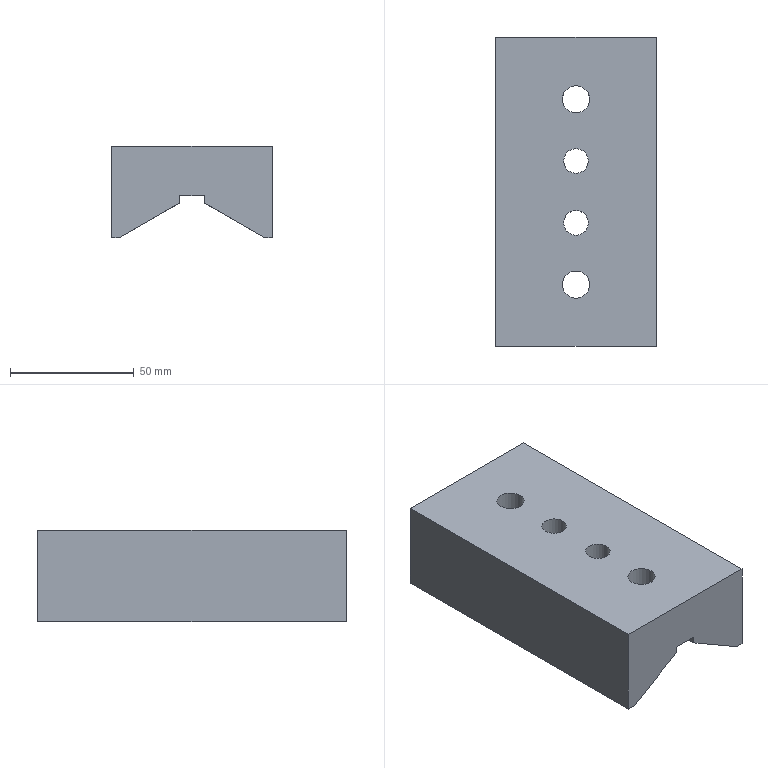Part | NX | features MAIN_BODY 2 | 1 solid | 34 faces | box 65 x 125 x 37 mm | volume 225809 mm3 | plane 24 | cylinder 10 | commonest cylinder face diameters 11 x6 10 x2 17.5 x2
STEP:
#1=CARTESIAN_POINT('',(420.,435.,-240.));
#2=VERTEX_POINT('',#1);
#3=CARTESIAN_POINT('',(420.,452.819,-240.));
#4=VERTEX_POINT('',#3);
#5=CARTESIAN_POINT('',(420.,435.,-240.));
#6=DIRECTION('',(0.,1.,0.));
#7=VECTOR('',#6,1000.);
#8=LINE('',#5,#7);
#9=EDGE_CURVE('',#2,#4,#8,.T.);
#10=ORIENTED_EDGE('',*,*,#9,.T.);
#11=CARTESIAN_POINT('',(430.,452.819,-240.));
#12=VERTEX_POINT('',#11);
#13=CARTESIAN_POINT('',(425.,460.,-240.));
#14=DIRECTION('',(0.,0.,1.));
#15=DIRECTION('',(-1.,0.,0.));
#16=AXIS2_PLACEMENT_3D('',#13,#14,#15);
#17=CIRCLE('',#16,8.75);
#18=EDGE_CURVE('',#4,#12,#17,.T.);
#19=ORIENTED_EDGE('',*,*,#18,.T.);
#20=CARTESIAN_POINT('',(430.,435.,-240.));
#21=VERTEX_POINT('',#20);
#22=CARTESIAN_POINT('',(430.,435.,-240.));
#23=DIRECTION('',(0.,1.,0.));
#24=VECTOR('',#23,1000.);
#25=LINE('',#22,#24);
#26=EDGE_CURVE('',#21,#12,#25,.T.);
#27=ORIENTED_EDGE('',*,*,#26,.F.);
#28=CARTESIAN_POINT('',(430.,435.,-240.));
#29=DIRECTION('',(-1.,0.,0.));
#30=VECTOR('',#29,1000.);
#31=LINE('',#28,#30);
#32=EDGE_CURVE('',#21,#2,#31,.T.);
#33=ORIENTED_EDGE('',*,*,#32,.T.);
#34=EDGE_LOOP('',(#10,#19,#27,#33));
#35=FACE_BOUND('',#34,.T.);
#36=CARTESIAN_POINT('',(420.,435.,-240.));
#37=DIRECTION('',(0.,0.,1.));
#38=DIRECTION('',(-1.,0.,0.));
#39=AXIS2_PLACEMENT_3D('',#36,#37,#38);
#40=PLANE('',#39);
#41=ADVANCED_FACE('',(#35),#40,.F.);
#42=CARTESIAN_POINT('',(430.,452.819,-242.887));
#43=VERTEX_POINT('',#42);
#44=CARTESIAN_POINT('',(430.,452.819,-250.));
#45=DIRECTION('',(0.,0.,1.));
#46=VECTOR('',#45,1000.);
#47=LINE('',#44,#46);
#48=EDGE_CURVE('',#43,#12,#47,.T.);
#49=ORIENTED_EDGE('',*,*,#48,.F.);
#50=CARTESIAN_POINT('',(430.,435.,-242.887));
#51=VERTEX_POINT('',#50);
#52=CARTESIAN_POINT('',(430.,435.,-242.887));
#53=DIRECTION('',(0.,1.,0.));
#54=VECTOR('',#53,1000.);
#55=LINE('',#52,#54);
#56=EDGE_CURVE('',#51,#43,#55,.T.);
#57=ORIENTED_EDGE('',*,*,#56,.F.);
#58=CARTESIAN_POINT('',(430.,435.,-242.887));
#59=DIRECTION('',(0.,0.,1.));
#60=VECTOR('',#59,1000.);
#61=LINE('',#58,#60);
#62=EDGE_CURVE('',#51,#21,#61,.T.);
#63=ORIENTED_EDGE('',*,*,#62,.T.);
#64=ORIENTED_EDGE('',*,*,#26,.T.);
#65=EDGE_LOOP('',(#49,#57,#63,#64));
#66=FACE_BOUND('',#65,.T.);
#67=CARTESIAN_POINT('',(430.,435.,-242.887));
#68=DIRECTION('',(-1.,0.,0.));
#69=DIRECTION('',(0.,0.,-1.));
#70=AXIS2_PLACEMENT_3D('',#67,#68,#69);
#71=PLANE('',#70);
#72=ADVANCED_FACE('',(#66),#71,.T.);
#73=CARTESIAN_POINT('',(420.,435.,-242.887));
#74=VERTEX_POINT('',#73);
#75=CARTESIAN_POINT('',(420.,452.819,-242.887));
#76=VERTEX_POINT('',#75);
#77=CARTESIAN_POINT('',(420.,435.,-242.887));
#78=DIRECTION('',(0.,1.,0.));
#79=VECTOR('',#78,1000.);
#80=LINE('',#77,#79);
#81=EDGE_CURVE('',#74,#76,#80,.T.);
#82=ORIENTED_EDGE('',*,*,#81,.T.);
#83=CARTESIAN_POINT('',(420.,452.819,-250.));
#84=DIRECTION('',(0.,0.,1.));
#85=VECTOR('',#84,1000.);
#86=LINE('',#83,#85);
#87=EDGE_CURVE('',#76,#4,#86,.T.);
#88=ORIENTED_EDGE('',*,*,#87,.T.);
#89=ORIENTED_EDGE('',*,*,#9,.F.);
#90=CARTESIAN_POINT('',(420.,435.,-242.887));
#91=DIRECTION('',(0.,0.,1.));
#92=VECTOR('',#91,1000.);
#93=LINE('',#90,#92);
#94=EDGE_CURVE('',#74,#2,#93,.T.);
#95=ORIENTED_EDGE('',*,*,#94,.F.);
#96=EDGE_LOOP('',(#82,#88,#89,#95));
#97=FACE_BOUND('',#96,.T.);
#98=CARTESIAN_POINT('',(420.,435.,-242.887));
#99=DIRECTION('',(-1.,0.,0.));
#100=DIRECTION('',(0.,0.,-1.));
#101=AXIS2_PLACEMENT_3D('',#98,#99,#100);
#102=PLANE('',#101);
#103=ADVANCED_FACE('',(#97),#102,.F.);
#104=CARTESIAN_POINT('',(430.,467.181,-242.887));
#105=VERTEX_POINT('',#104);
#106=CARTESIAN_POINT('',(425.,460.,-240.));
#107=DIRECTION('',(-0.5,0.,-0.866));
#108=DIRECTION('',(-0.866,0.,0.5));
#109=AXIS2_PLACEMENT_3D('',#106,#107,#108);
#110=ELLIPSE('',#109,10.104,8.75);
#111=EDGE_CURVE('',#105,#43,#110,.T.);
#112=ORIENTED_EDGE('',*,*,#111,.F.);
#113=CARTESIAN_POINT('',(430.,482.709,-242.887));
#114=VERTEX_POINT('',#113);
#115=CARTESIAN_POINT('',(430.,435.,-242.887));
#116=DIRECTION('',(0.,1.,0.));
#117=VECTOR('',#116,1000.);
#118=LINE('',#115,#117);
#119=EDGE_CURVE('',#105,#114,#118,.T.);
#120=ORIENTED_EDGE('',*,*,#119,.T.);
#121=CARTESIAN_POINT('',(430.,487.291,-242.887));
#122=VERTEX_POINT('',#121);
#123=CARTESIAN_POINT('',(425.,485.,-240.));
#124=DIRECTION('',(-0.5,0.,-0.866));
#125=DIRECTION('',(0.866,0.,-0.5));
#126=AXIS2_PLACEMENT_3D('',#123,#124,#125);
#127=ELLIPSE('',#126,6.351,5.5);
#128=EDGE_CURVE('',#114,#122,#127,.F.);
#129=ORIENTED_EDGE('',*,*,#128,.T.);
#130=CARTESIAN_POINT('',(430.,507.709,-242.887));
#131=VERTEX_POINT('',#130);
#132=CARTESIAN_POINT('',(430.,435.,-242.887));
#133=DIRECTION('',(0.,1.,0.));
#134=VECTOR('',#133,1000.);
#135=LINE('',#132,#134);
#136=EDGE_CURVE('',#122,#131,#135,.T.);
#137=ORIENTED_EDGE('',*,*,#136,.T.);
#138=CARTESIAN_POINT('',(430.,512.291,-242.887));
#139=VERTEX_POINT('',#138);
#140=CARTESIAN_POINT('',(425.,510.,-240.));
#141=DIRECTION('',(-0.5,0.,-0.866));
#142=DIRECTION('',(0.866,0.,-0.5));
#143=AXIS2_PLACEMENT_3D('',#140,#141,#142);
#144=ELLIPSE('',#143,6.351,5.5);
#145=EDGE_CURVE('',#131,#139,#144,.F.);
#146=ORIENTED_EDGE('',*,*,#145,.T.);
#147=CARTESIAN_POINT('',(430.,527.819,-242.887));
#148=VERTEX_POINT('',#147);
#149=CARTESIAN_POINT('',(430.,435.,-242.887));
#150=DIRECTION('',(0.,1.,0.));
#151=VECTOR('',#150,1000.);
#152=LINE('',#149,#151);
#153=EDGE_CURVE('',#139,#148,#152,.T.);
#154=ORIENTED_EDGE('',*,*,#153,.T.);
#155=CARTESIAN_POINT('',(430.,542.181,-242.887));
#156=VERTEX_POINT('',#155);
#157=CARTESIAN_POINT('',(425.,535.,-240.));
#158=DIRECTION('',(-0.5,0.,-0.866));
#159=DIRECTION('',(-0.866,0.,0.5));
#160=AXIS2_PLACEMENT_3D('',#157,#158,#159);
#161=ELLIPSE('',#160,10.104,8.75);
#162=EDGE_CURVE('',#148,#156,#161,.F.);
#163=ORIENTED_EDGE('',*,*,#162,.T.);
#164=CARTESIAN_POINT('',(430.,560.,-242.887));
#165=VERTEX_POINT('',#164);
#166=CARTESIAN_POINT('',(430.,435.,-242.887));
#167=DIRECTION('',(0.,1.,0.));
#168=VECTOR('',#167,1000.);
#169=LINE('',#166,#168);
#170=EDGE_CURVE('',#156,#165,#169,.T.);
#171=ORIENTED_EDGE('',*,*,#170,.T.);
#172=CARTESIAN_POINT('',(454.445,560.,-257.));
#173=VERTEX_POINT('',#172);
#174=CARTESIAN_POINT('',(454.445,560.,-257.));
#175=DIRECTION('',(-0.866,0.,0.5));
#176=VECTOR('',#175,1000.);
#177=LINE('',#174,#176);
#178=EDGE_CURVE('',#173,#165,#177,.T.);
#179=ORIENTED_EDGE('',*,*,#178,.F.);
#180=CARTESIAN_POINT('',(454.445,435.,-257.));
#181=VERTEX_POINT('',#180);
#182=CARTESIAN_POINT('',(454.445,435.,-257.));
#183=DIRECTION('',(0.,1.,0.));
#184=VECTOR('',#183,1000.);
#185=LINE('',#182,#184);
#186=EDGE_CURVE('',#181,#173,#185,.T.);
#187=ORIENTED_EDGE('',*,*,#186,.F.);
#188=CARTESIAN_POINT('',(454.445,435.,-257.));
#189=DIRECTION('',(-0.866,0.,0.5));
#190=VECTOR('',#189,1000.);
#191=LINE('',#188,#190);
#192=EDGE_CURVE('',#181,#51,#191,.T.);
#193=ORIENTED_EDGE('',*,*,#192,.T.);
#194=ORIENTED_EDGE('',*,*,#56,.T.);
#195=EDGE_LOOP('',(#112,#120,#129,#137,#146,#154,#163,#171,#179,#187,#193,#194));
#196=FACE_BOUND('',#195,.T.);
#197=CARTESIAN_POINT('',(454.445,435.,-257.));
#198=DIRECTION('',(-0.5,0.,-0.866));
#199=DIRECTION('',(0.866,0.,-0.5));
#200=AXIS2_PLACEMENT_3D('',#197,#198,#199);
#201=PLANE('',#200);
#202=ADVANCED_FACE('',(#196),#201,.T.);
#203=CARTESIAN_POINT('',(430.,512.291,-240.));
#204=VERTEX_POINT('',#203);
#205=CARTESIAN_POINT('',(430.,527.819,-240.));
#206=VERTEX_POINT('',#205);
#207=CARTESIAN_POINT('',(430.,435.,-240.));
#208=DIRECTION('',(0.,1.,0.));
#209=VECTOR('',#208,1000.);
#210=LINE('',#207,#209);
#211=EDGE_CURVE('',#204,#206,#210,.T.);
#212=ORIENTED_EDGE('',*,*,#211,.T.);
#213=CARTESIAN_POINT('',(430.,527.819,-250.));
#214=DIRECTION('',(0.,0.,1.));
#215=VECTOR('',#214,1000.);
#216=LINE('',#213,#215);
#217=EDGE_CURVE('',#206,#148,#216,.F.);
#218=ORIENTED_EDGE('',*,*,#217,.T.);
#219=ORIENTED_EDGE('',*,*,#153,.F.);
#220=CARTESIAN_POINT('',(430.,512.291,-240.));
#221=DIRECTION('',(0.,0.,-1.));
#222=VECTOR('',#221,1000.);
#223=LINE('',#220,#222);
#224=EDGE_CURVE('',#139,#204,#223,.F.);
#225=ORIENTED_EDGE('',*,*,#224,.T.);
#226=EDGE_LOOP('',(#212,#218,#219,#225));
#227=FACE_BOUND('',#226,.T.);
#228=CARTESIAN_POINT('',(430.,435.,-242.887));
#229=DIRECTION('',(-1.,0.,0.));
#230=DIRECTION('',(0.,0.,-1.));
#231=AXIS2_PLACEMENT_3D('',#228,#229,#230);
#232=PLANE('',#231);
#233=ADVANCED_FACE('',(#227),#232,.T.);
#234=ORIENTED_EDGE('',*,*,#170,.F.);
#235=CARTESIAN_POINT('',(430.,542.181,-240.));
#236=VERTEX_POINT('',#235);
#237=CARTESIAN_POINT('',(430.,542.181,-250.));
#238=DIRECTION('',(0.,0.,1.));
#239=VECTOR('',#238,1000.);
#240=LINE('',#237,#239);
#241=EDGE_CURVE('',#156,#236,#240,.T.);
#242=ORIENTED_EDGE('',*,*,#241,.T.);
#243=CARTESIAN_POINT('',(430.,560.,-240.));
#244=VERTEX_POINT('',#243);
#245=CARTESIAN_POINT('',(430.,435.,-240.));
#246=DIRECTION('',(0.,1.,0.));
#247=VECTOR('',#246,1000.);
#248=LINE('',#245,#247);
#249=EDGE_CURVE('',#236,#244,#248,.T.);
#250=ORIENTED_EDGE('',*,*,#249,.T.);
#251=CARTESIAN_POINT('',(430.,560.,-242.887));
#252=DIRECTION('',(0.,0.,1.));
#253=VECTOR('',#252,1000.);
#254=LINE('',#251,#253);
#255=EDGE_CURVE('',#165,#244,#254,.T.);
#256=ORIENTED_EDGE('',*,*,#255,.F.);
#257=EDGE_LOOP('',(#234,#242,#250,#256));
#258=FACE_BOUND('',#257,.T.);
#259=CARTESIAN_POINT('',(430.,435.,-242.887));
#260=DIRECTION('',(-1.,0.,0.));
#261=DIRECTION('',(0.,0.,-1.));
#262=AXIS2_PLACEMENT_3D('',#259,#260,#261);
#263=PLANE('',#262);
#264=ADVANCED_FACE('',(#258),#263,.T.);
#265=CARTESIAN_POINT('',(420.,527.819,-240.));
#266=VERTEX_POINT('',#265);
#267=CARTESIAN_POINT('',(420.,527.819,-242.887));
#268=VERTEX_POINT('',#267);
#269=CARTESIAN_POINT('',(420.,527.819,-250.));
#270=DIRECTION('',(0.,0.,1.));
#271=VECTOR('',#270,1000.);
#272=LINE('',#269,#271);
#273=EDGE_CURVE('',#266,#268,#272,.F.);
#274=ORIENTED_EDGE('',*,*,#273,.F.);
#275=CARTESIAN_POINT('',(420.,512.291,-240.));
#276=VERTEX_POINT('',#275);
#277=CARTESIAN_POINT('',(420.,435.,-240.));
#278=DIRECTION('',(0.,1.,0.));
#279=VECTOR('',#278,1000.);
#280=LINE('',#277,#279);
#281=EDGE_CURVE('',#276,#266,#280,.T.);
#282=ORIENTED_EDGE('',*,*,#281,.F.);
#283=CARTESIAN_POINT('',(420.,512.291,-242.887));
#284=VERTEX_POINT('',#283);
#285=CARTESIAN_POINT('',(420.,512.291,-240.));
#286=DIRECTION('',(0.,0.,-1.));
#287=VECTOR('',#286,1000.);
#288=LINE('',#285,#287);
#289=EDGE_CURVE('',#284,#276,#288,.F.);
#290=ORIENTED_EDGE('',*,*,#289,.F.);
#291=CARTESIAN_POINT('',(420.,435.,-242.887));
#292=DIRECTION('',(0.,1.,0.));
#293=VECTOR('',#292,1000.);
#294=LINE('',#291,#293);
#295=EDGE_CURVE('',#284,#268,#294,.T.);
#296=ORIENTED_EDGE('',*,*,#295,.T.);
#297=EDGE_LOOP('',(#274,#282,#290,#296));
#298=FACE_BOUND('',#297,.T.);
#299=CARTESIAN_POINT('',(420.,435.,-242.887));
#300=DIRECTION('',(-1.,0.,0.));
#301=DIRECTION('',(0.,0.,-1.));
#302=AXIS2_PLACEMENT_3D('',#299,#300,#301);
#303=PLANE('',#302);
#304=ADVANCED_FACE('',(#298),#303,.F.);
#305=CARTESIAN_POINT('',(420.,542.181,-242.887));
#306=VERTEX_POINT('',#305);
#307=CARTESIAN_POINT('',(420.,542.181,-240.));
#308=VERTEX_POINT('',#307);
#309=CARTESIAN_POINT('',(420.,542.181,-250.));
#310=DIRECTION('',(0.,0.,1.));
#311=VECTOR('',#310,1000.);
#312=LINE('',#309,#311);
#313=EDGE_CURVE('',#306,#308,#312,.T.);
#314=ORIENTED_EDGE('',*,*,#313,.F.);
#315=CARTESIAN_POINT('',(420.,560.,-242.887));
#316=VERTEX_POINT('',#315);
#317=CARTESIAN_POINT('',(420.,435.,-242.887));
#318=DIRECTION('',(0.,1.,0.));
#319=VECTOR('',#318,1000.);
#320=LINE('',#317,#319);
#321=EDGE_CURVE('',#306,#316,#320,.T.);
#322=ORIENTED_EDGE('',*,*,#321,.T.);
#323=CARTESIAN_POINT('',(420.,560.,-240.));
#324=VERTEX_POINT('',#323);
#325=CARTESIAN_POINT('',(420.,560.,-242.887));
#326=DIRECTION('',(0.,0.,1.));
#327=VECTOR('',#326,1000.);
#328=LINE('',#325,#327);
#329=EDGE_CURVE('',#316,#324,#328,.T.);
#330=ORIENTED_EDGE('',*,*,#329,.T.);
#331=CARTESIAN_POINT('',(420.,435.,-240.));
#332=DIRECTION('',(0.,1.,0.));
#333=VECTOR('',#332,1000.);
#334=LINE('',#331,#333);
#335=EDGE_CURVE('',#308,#324,#334,.T.);
#336=ORIENTED_EDGE('',*,*,#335,.F.);
#337=EDGE_LOOP('',(#314,#322,#330,#336));
#338=FACE_BOUND('',#337,.T.);
#339=CARTESIAN_POINT('',(420.,435.,-242.887));
#340=DIRECTION('',(-1.,0.,0.));
#341=DIRECTION('',(0.,0.,-1.));
#342=AXIS2_PLACEMENT_3D('',#339,#340,#341);
#343=PLANE('',#342);
#344=ADVANCED_FACE('',(#338),#343,.F.);
#345=CARTESIAN_POINT('',(420.,467.181,-242.887));
#346=VERTEX_POINT('',#345);
#347=CARTESIAN_POINT('',(420.,482.709,-242.887));
#348=VERTEX_POINT('',#347);
#349=CARTESIAN_POINT('',(420.,435.,-242.887));
#350=DIRECTION('',(0.,1.,0.));
#351=VECTOR('',#350,1000.);
#352=LINE('',#349,#351);
#353=EDGE_CURVE('',#346,#348,#352,.T.);
#354=ORIENTED_EDGE('',*,*,#353,.F.);
#355=CARTESIAN_POINT('',(425.,460.,-240.));
#356=DIRECTION('',(-0.5,0.,0.866));
#357=DIRECTION('',(0.866,0.,0.5));
#358=AXIS2_PLACEMENT_3D('',#355,#356,#357);
#359=ELLIPSE('',#358,10.104,8.75);
#360=EDGE_CURVE('',#346,#76,#359,.T.);
#361=ORIENTED_EDGE('',*,*,#360,.T.);
#362=ORIENTED_EDGE('',*,*,#81,.F.);
#363=CARTESIAN_POINT('',(395.555,435.,-257.));
#364=VERTEX_POINT('',#363);
#365=CARTESIAN_POINT('',(395.555,435.,-257.));
#366=DIRECTION('',(0.866,0.,0.5));
#367=VECTOR('',#366,1000.);
#368=LINE('',#365,#367);
#369=EDGE_CURVE('',#364,#74,#368,.T.);
#370=ORIENTED_EDGE('',*,*,#369,.F.);
#371=CARTESIAN_POINT('',(395.555,560.,-257.));
#372=VERTEX_POINT('',#371);
#373=CARTESIAN_POINT('',(395.555,435.,-257.));
#374=DIRECTION('',(0.,1.,0.));
#375=VECTOR('',#374,1000.);
#376=LINE('',#373,#375);
#377=EDGE_CURVE('',#364,#372,#376,.T.);
#378=ORIENTED_EDGE('',*,*,#377,.T.);
#379=CARTESIAN_POINT('',(395.555,560.,-257.));
#380=DIRECTION('',(0.866,0.,0.5));
#381=VECTOR('',#380,1000.);
#382=LINE('',#379,#381);
#383=EDGE_CURVE('',#372,#316,#382,.T.);
#384=ORIENTED_EDGE('',*,*,#383,.T.);
#385=ORIENTED_EDGE('',*,*,#321,.F.);
#386=CARTESIAN_POINT('',(425.,535.,-240.));
#387=DIRECTION('',(-0.5,0.,0.866));
#388=DIRECTION('',(0.866,0.,0.5));
#389=AXIS2_PLACEMENT_3D('',#386,#387,#388);
#390=ELLIPSE('',#389,10.104,8.75);
#391=EDGE_CURVE('',#268,#306,#390,.F.);
#392=ORIENTED_EDGE('',*,*,#391,.F.);
#393=ORIENTED_EDGE('',*,*,#295,.F.);
#394=CARTESIAN_POINT('',(420.,507.709,-242.887));
#395=VERTEX_POINT('',#394);
#396=CARTESIAN_POINT('',(425.,510.,-240.));
#397=DIRECTION('',(-0.5,0.,0.866));
#398=DIRECTION('',(-0.866,0.,-0.5));
#399=AXIS2_PLACEMENT_3D('',#396,#397,#398);
#400=ELLIPSE('',#399,6.351,5.5);
#401=EDGE_CURVE('',#395,#284,#400,.F.);
#402=ORIENTED_EDGE('',*,*,#401,.F.);
#403=CARTESIAN_POINT('',(420.,487.291,-242.887));
#404=VERTEX_POINT('',#403);
#405=CARTESIAN_POINT('',(420.,435.,-242.887));
#406=DIRECTION('',(0.,1.,0.));
#407=VECTOR('',#406,1000.);
#408=LINE('',#405,#407);
#409=EDGE_CURVE('',#404,#395,#408,.T.);
#410=ORIENTED_EDGE('',*,*,#409,.F.);
#411=CARTESIAN_POINT('',(425.,485.,-240.));
#412=DIRECTION('',(-0.5,0.,0.866));
#413=DIRECTION('',(-0.866,0.,-0.5));
#414=AXIS2_PLACEMENT_3D('',#411,#412,#413);
#415=ELLIPSE('',#414,6.351,5.5);
#416=EDGE_CURVE('',#348,#404,#415,.F.);
#417=ORIENTED_EDGE('',*,*,#416,.F.);
#418=EDGE_LOOP('',(#354,#361,#362,#370,#378,#384,#385,#392,#393,#402,#410,#417));
#419=FACE_BOUND('',#418,.T.);
#420=CARTESIAN_POINT('',(395.555,435.,-257.));
#421=DIRECTION('',(-0.5,0.,0.866));
#422=DIRECTION('',(-0.866,0.,-0.5));
#423=AXIS2_PLACEMENT_3D('',#420,#421,#422);
#424=PLANE('',#423);
#425=ADVANCED_FACE('',(#419),#424,.F.);
#426=CARTESIAN_POINT('',(425.,535.,-240.));
#427=DIRECTION('',(0.,0.,1.));
#428=DIRECTION('',(-1.,0.,0.));
#429=AXIS2_PLACEMENT_3D('',#426,#427,#428);
#430=CIRCLE('',#429,8.75);
#431=EDGE_CURVE('',#308,#236,#430,.F.);
#432=ORIENTED_EDGE('',*,*,#431,.F.);
#433=ORIENTED_EDGE('',*,*,#335,.T.);
#434=CARTESIAN_POINT('',(420.,560.,-240.));
#435=DIRECTION('',(1.,0.,0.));
#436=VECTOR('',#435,1000.);
#437=LINE('',#434,#436);
#438=EDGE_CURVE('',#324,#244,#437,.T.);
#439=ORIENTED_EDGE('',*,*,#438,.T.);
#440=ORIENTED_EDGE('',*,*,#249,.F.);
#441=EDGE_LOOP('',(#432,#433,#439,#440));
#442=FACE_BOUND('',#441,.T.);
#443=CARTESIAN_POINT('',(420.,435.,-240.));
#444=DIRECTION('',(0.,0.,1.));
#445=DIRECTION('',(-1.,0.,0.));
#446=AXIS2_PLACEMENT_3D('',#443,#444,#445);
#447=PLANE('',#446);
#448=ADVANCED_FACE('',(#442),#447,.F.);
#449=CARTESIAN_POINT('',(430.,485.,-240.));
#450=VERTEX_POINT('',#449);
#451=CARTESIAN_POINT('',(425.,485.,-240.));
#452=DIRECTION('',(0.,0.,-1.));
#453=DIRECTION('',(1.,0.,0.));
#454=AXIS2_PLACEMENT_3D('',#451,#452,#453);
#455=CIRCLE('',#454,5.);
#456=EDGE_CURVE('',#450,#450,#455,.T.);
#457=ORIENTED_EDGE('',*,*,#456,.F.);
#458=EDGE_LOOP('',(#457));
#459=FACE_BOUND('',#458,.T.);
#460=CARTESIAN_POINT('',(430.,510.,-240.));
#461=VERTEX_POINT('',#460);
#462=CARTESIAN_POINT('',(425.,510.,-240.));
#463=DIRECTION('',(0.,0.,-1.));
#464=DIRECTION('',(1.,0.,0.));
#465=AXIS2_PLACEMENT_3D('',#462,#463,#464);
#466=CIRCLE('',#465,5.);
#467=EDGE_CURVE('',#461,#461,#466,.T.);
#468=ORIENTED_EDGE('',*,*,#467,.F.);
#469=EDGE_LOOP('',(#468));
#470=FACE_BOUND('',#469,.T.);
#471=CARTESIAN_POINT('',(430.,467.181,-240.));
#472=VERTEX_POINT('',#471);
#473=CARTESIAN_POINT('',(430.,482.709,-240.));
#474=VERTEX_POINT('',#473);
#475=CARTESIAN_POINT('',(430.,435.,-240.));
#476=DIRECTION('',(0.,1.,0.));
#477=VECTOR('',#476,1000.);
#478=LINE('',#475,#477);
#479=EDGE_CURVE('',#472,#474,#478,.T.);
#480=ORIENTED_EDGE('',*,*,#479,.F.);
#481=CARTESIAN_POINT('',(420.,467.181,-240.));
#482=VERTEX_POINT('',#481);
#483=CARTESIAN_POINT('',(425.,460.,-240.));
#484=DIRECTION('',(0.,0.,1.));
#485=DIRECTION('',(-1.,0.,0.));
#486=AXIS2_PLACEMENT_3D('',#483,#484,#485);
#487=CIRCLE('',#486,8.75);
#488=EDGE_CURVE('',#472,#482,#487,.T.);
#489=ORIENTED_EDGE('',*,*,#488,.T.);
#490=CARTESIAN_POINT('',(420.,482.709,-240.));
#491=VERTEX_POINT('',#490);
#492=CARTESIAN_POINT('',(420.,435.,-240.));
#493=DIRECTION('',(0.,1.,0.));
#494=VECTOR('',#493,1000.);
#495=LINE('',#492,#494);
#496=EDGE_CURVE('',#482,#491,#495,.T.);
#497=ORIENTED_EDGE('',*,*,#496,.T.);
#498=CARTESIAN_POINT('',(420.,487.291,-240.));
#499=VERTEX_POINT('',#498);
#500=CARTESIAN_POINT('',(425.,485.,-240.));
#501=DIRECTION('',(0.,0.,-1.));
#502=DIRECTION('',(1.,0.,0.));
#503=AXIS2_PLACEMENT_3D('',#500,#501,#502);
#504=CIRCLE('',#503,5.5);
#505=EDGE_CURVE('',#499,#491,#504,.F.);
#506=ORIENTED_EDGE('',*,*,#505,.F.);
#507=CARTESIAN_POINT('',(420.,507.709,-240.));
#508=VERTEX_POINT('',#507);
#509=CARTESIAN_POINT('',(420.,435.,-240.));
#510=DIRECTION('',(0.,1.,0.));
#511=VECTOR('',#510,1000.);
#512=LINE('',#509,#511);
#513=EDGE_CURVE('',#499,#508,#512,.T.);
#514=ORIENTED_EDGE('',*,*,#513,.T.);
#515=CARTESIAN_POINT('',(425.,510.,-240.));
#516=DIRECTION('',(0.,0.,-1.));
#517=DIRECTION('',(1.,0.,0.));
#518=AXIS2_PLACEMENT_3D('',#515,#516,#517);
#519=CIRCLE('',#518,5.5);
#520=EDGE_CURVE('',#276,#508,#519,.F.);
#521=ORIENTED_EDGE('',*,*,#520,.F.);
#522=ORIENTED_EDGE('',*,*,#281,.T.);
#523=CARTESIAN_POINT('',(425.,535.,-240.));
#524=DIRECTION('',(0.,0.,1.));
#525=DIRECTION('',(-1.,0.,0.));
#526=AXIS2_PLACEMENT_3D('',#523,#524,#525);
#527=CIRCLE('',#526,8.75);
#528=EDGE_CURVE('',#206,#266,#527,.F.);
#529=ORIENTED_EDGE('',*,*,#528,.F.);
#530=ORIENTED_EDGE('',*,*,#211,.F.);
#531=CARTESIAN_POINT('',(430.,507.709,-240.));
#532=VERTEX_POINT('',#531);
#533=CARTESIAN_POINT('',(425.,510.,-240.));
#534=DIRECTION('',(0.,0.,-1.));
#535=DIRECTION('',(1.,0.,0.));
#536=AXIS2_PLACEMENT_3D('',#533,#534,#535);
#537=CIRCLE('',#536,5.5);
#538=EDGE_CURVE('',#532,#204,#537,.F.);
#539=ORIENTED_EDGE('',*,*,#538,.F.);
#540=CARTESIAN_POINT('',(430.,487.291,-240.));
#541=VERTEX_POINT('',#540);
#542=CARTESIAN_POINT('',(430.,435.,-240.));
#543=DIRECTION('',(0.,1.,0.));
#544=VECTOR('',#543,1000.);
#545=LINE('',#542,#544);
#546=EDGE_CURVE('',#541,#532,#545,.T.);
#547=ORIENTED_EDGE('',*,*,#546,.F.);
#548=CARTESIAN_POINT('',(425.,485.,-240.));
#549=DIRECTION('',(0.,0.,-1.));
#550=DIRECTION('',(1.,0.,0.));
#551=AXIS2_PLACEMENT_3D('',#548,#549,#550);
#552=CIRCLE('',#551,5.5);
#553=EDGE_CURVE('',#474,#541,#552,.F.);
#554=ORIENTED_EDGE('',*,*,#553,.F.);
#555=EDGE_LOOP('',(#480,#489,#497,#506,#514,#521,#522,#529,#530,#539,#547,#554));
#556=FACE_BOUND('',#555,.T.);
#557=CARTESIAN_POINT('',(420.,435.,-240.));
#558=DIRECTION('',(0.,0.,1.));
#559=DIRECTION('',(-1.,0.,0.));
#560=AXIS2_PLACEMENT_3D('',#557,#558,#559);
#561=PLANE('',#560);
#562=ADVANCED_FACE('',(#459,#470,#556),#561,.F.);
#563=CARTESIAN_POINT('',(430.5,460.,-220.));
#564=VERTEX_POINT('',#563);
#565=CARTESIAN_POINT('',(425.,460.,-220.));
#566=DIRECTION('',(0.,0.,1.));
#567=DIRECTION('',(1.,0.,0.));
#568=AXIS2_PLACEMENT_3D('',#565,#566,#567);
#569=CIRCLE('',#568,5.5);
#570=EDGE_CURVE('',#564,#564,#569,.T.);
#571=ORIENTED_EDGE('',*,*,#570,.F.);
#572=EDGE_LOOP('',(#571));
#573=FACE_BOUND('',#572,.T.);
#574=CARTESIAN_POINT('',(392.5,560.,-220.));
#575=VERTEX_POINT('',#574);
#576=CARTESIAN_POINT('',(457.5,560.,-220.));
#577=VERTEX_POINT('',#576);
#578=CARTESIAN_POINT('',(425.,560.,-220.));
#579=DIRECTION('',(1.,0.,0.));
#580=VECTOR('',#579,1000.);
#581=LINE('',#578,#580);
#582=EDGE_CURVE('',#575,#577,#581,.T.);
#583=ORIENTED_EDGE('',*,*,#582,.F.);
#584=CARTESIAN_POINT('',(392.5,435.,-220.));
#585=VERTEX_POINT('',#584);
#586=CARTESIAN_POINT('',(392.5,435.,-220.));
#587=DIRECTION('',(0.,1.,0.));
#588=VECTOR('',#587,1000.);
#589=LINE('',#586,#588);
#590=EDGE_CURVE('',#585,#575,#589,.T.);
#591=ORIENTED_EDGE('',*,*,#590,.F.);
#592=CARTESIAN_POINT('',(457.5,435.,-220.));
#593=VERTEX_POINT('',#592);
#594=CARTESIAN_POINT('',(425.,435.,-220.));
#595=DIRECTION('',(-1.,0.,0.));
#596=VECTOR('',#595,1000.);
#597=LINE('',#594,#596);
#598=EDGE_CURVE('',#593,#585,#597,.T.);
#599=ORIENTED_EDGE('',*,*,#598,.F.);
#600=CARTESIAN_POINT('',(457.5,435.,-220.));
#601=DIRECTION('',(0.,1.,0.));
#602=VECTOR('',#601,1000.);
#603=LINE('',#600,#602);
#604=EDGE_CURVE('',#593,#577,#603,.T.);
#605=ORIENTED_EDGE('',*,*,#604,.T.);
#606=EDGE_LOOP('',(#583,#591,#599,#605));
#607=FACE_BOUND('',#606,.T.);
#608=CARTESIAN_POINT('',(430.,485.,-220.));
#609=VERTEX_POINT('',#608);
#610=CARTESIAN_POINT('',(425.,485.,-220.));
#611=DIRECTION('',(0.,0.,-1.));
#612=DIRECTION('',(1.,0.,0.));
#613=AXIS2_PLACEMENT_3D('',#610,#611,#612);
#614=CIRCLE('',#613,5.);
#615=EDGE_CURVE('',#609,#609,#614,.T.);
#616=ORIENTED_EDGE('',*,*,#615,.T.);
#617=EDGE_LOOP('',(#616));
#618=FACE_BOUND('',#617,.T.);
#619=CARTESIAN_POINT('',(430.,510.,-220.));
#620=VERTEX_POINT('',#619);
#621=CARTESIAN_POINT('',(425.,510.,-220.));
#622=DIRECTION('',(0.,0.,-1.));
#623=DIRECTION('',(1.,0.,0.));
#624=AXIS2_PLACEMENT_3D('',#621,#622,#623);
#625=CIRCLE('',#624,5.);
#626=EDGE_CURVE('',#620,#620,#625,.T.);
#627=ORIENTED_EDGE('',*,*,#626,.T.);
#628=EDGE_LOOP('',(#627));
#629=FACE_BOUND('',#628,.T.);
#630=CARTESIAN_POINT('',(430.5,535.,-220.));
#631=VERTEX_POINT('',#630);
#632=CARTESIAN_POINT('',(425.,535.,-220.));
#633=DIRECTION('',(0.,0.,-1.));
#634=DIRECTION('',(1.,0.,0.));
#635=AXIS2_PLACEMENT_3D('',#632,#633,#634);
#636=CIRCLE('',#635,5.5);
#637=EDGE_CURVE('',#631,#631,#636,.T.);
#638=ORIENTED_EDGE('',*,*,#637,.T.);
#639=EDGE_LOOP('',(#638));
#640=FACE_BOUND('',#639,.T.);
#641=CARTESIAN_POINT('',(425.,435.,-220.));
#642=DIRECTION('',(0.,0.,1.));
#643=DIRECTION('',(-1.,0.,0.));
#644=AXIS2_PLACEMENT_3D('',#641,#642,#643);
#645=PLANE('',#644);
#646=ADVANCED_FACE('',(#573,#607,#618,#629,#640),#645,.T.);
#647=ORIENTED_EDGE('',*,*,#546,.T.);
#648=CARTESIAN_POINT('',(430.,507.709,-240.));
#649=DIRECTION('',(0.,0.,-1.));
#650=VECTOR('',#649,1000.);
#651=LINE('',#648,#650);
#652=EDGE_CURVE('',#532,#131,#651,.T.);
#653=ORIENTED_EDGE('',*,*,#652,.T.);
#654=ORIENTED_EDGE('',*,*,#136,.F.);
#655=CARTESIAN_POINT('',(430.,487.291,-240.));
#656=DIRECTION('',(0.,0.,-1.));
#657=VECTOR('',#656,1000.);
#658=LINE('',#655,#657);
#659=EDGE_CURVE('',#122,#541,#658,.F.);
#660=ORIENTED_EDGE('',*,*,#659,.T.);
#661=EDGE_LOOP('',(#647,#653,#654,#660));
#662=FACE_BOUND('',#661,.T.);
#663=CARTESIAN_POINT('',(430.,435.,-242.887));
#664=DIRECTION('',(-1.,0.,0.));
#665=DIRECTION('',(0.,0.,-1.));
#666=AXIS2_PLACEMENT_3D('',#663,#664,#665);
#667=PLANE('',#666);
#668=ADVANCED_FACE('',(#662),#667,.T.);
#669=CARTESIAN_POINT('',(420.,507.709,-240.));
#670=DIRECTION('',(0.,0.,-1.));
#671=VECTOR('',#670,1000.);
#672=LINE('',#669,#671);
#673=EDGE_CURVE('',#508,#395,#672,.T.);
#674=ORIENTED_EDGE('',*,*,#673,.F.);
#675=ORIENTED_EDGE('',*,*,#513,.F.);
#676=CARTESIAN_POINT('',(420.,487.291,-240.));
#677=DIRECTION('',(0.,0.,-1.));
#678=VECTOR('',#677,1000.);
#679=LINE('',#676,#678);
#680=EDGE_CURVE('',#404,#499,#679,.F.);
#681=ORIENTED_EDGE('',*,*,#680,.F.);
#682=ORIENTED_EDGE('',*,*,#409,.T.);
#683=EDGE_LOOP('',(#674,#675,#681,#682));
#684=FACE_BOUND('',#683,.T.);
#685=CARTESIAN_POINT('',(420.,435.,-242.887));
#686=DIRECTION('',(-1.,0.,0.));
#687=DIRECTION('',(0.,0.,-1.));
#688=AXIS2_PLACEMENT_3D('',#685,#686,#687);
#689=PLANE('',#688);
#690=ADVANCED_FACE('',(#684),#689,.F.);
#691=CARTESIAN_POINT('',(430.,467.181,-250.));
#692=DIRECTION('',(0.,0.,1.));
#693=VECTOR('',#692,1000.);
#694=LINE('',#691,#693);
#695=EDGE_CURVE('',#472,#105,#694,.F.);
#696=ORIENTED_EDGE('',*,*,#695,.F.);
#697=ORIENTED_EDGE('',*,*,#479,.T.);
#698=CARTESIAN_POINT('',(430.,482.709,-240.));
#699=DIRECTION('',(0.,0.,-1.));
#700=VECTOR('',#699,1000.);
#701=LINE('',#698,#700);
#702=EDGE_CURVE('',#474,#114,#701,.T.);
#703=ORIENTED_EDGE('',*,*,#702,.T.);
#704=ORIENTED_EDGE('',*,*,#119,.F.);
#705=EDGE_LOOP('',(#696,#697,#703,#704));
#706=FACE_BOUND('',#705,.T.);
#707=CARTESIAN_POINT('',(430.,435.,-242.887));
#708=DIRECTION('',(-1.,0.,0.));
#709=DIRECTION('',(0.,0.,-1.));
#710=AXIS2_PLACEMENT_3D('',#707,#708,#709);
#711=PLANE('',#710);
#712=ADVANCED_FACE('',(#706),#711,.T.);
#713=ORIENTED_EDGE('',*,*,#496,.F.);
#714=CARTESIAN_POINT('',(420.,467.181,-250.));
#715=DIRECTION('',(0.,0.,1.));
#716=VECTOR('',#715,1000.);
#717=LINE('',#714,#716);
#718=EDGE_CURVE('',#482,#346,#717,.F.);
#719=ORIENTED_EDGE('',*,*,#718,.T.);
#720=ORIENTED_EDGE('',*,*,#353,.T.);
#721=CARTESIAN_POINT('',(420.,482.709,-240.));
#722=DIRECTION('',(0.,0.,-1.));
#723=VECTOR('',#722,1000.);
#724=LINE('',#721,#723);
#725=EDGE_CURVE('',#491,#348,#724,.T.);
#726=ORIENTED_EDGE('',*,*,#725,.F.);
#727=EDGE_LOOP('',(#713,#719,#720,#726));
#728=FACE_BOUND('',#727,.T.);
#729=CARTESIAN_POINT('',(420.,435.,-242.887));
#730=DIRECTION('',(-1.,0.,0.));
#731=DIRECTION('',(0.,0.,-1.));
#732=AXIS2_PLACEMENT_3D('',#729,#730,#731);
#733=PLANE('',#732);
#734=ADVANCED_FACE('',(#728),#733,.F.);
#735=CARTESIAN_POINT('',(457.5,560.,-257.));
#736=VERTEX_POINT('',#735);
#737=CARTESIAN_POINT('',(457.5,560.,-257.));
#738=DIRECTION('',(-1.,0.,0.));
#739=VECTOR('',#738,1000.);
#740=LINE('',#737,#739);
#741=EDGE_CURVE('',#736,#173,#740,.T.);
#742=ORIENTED_EDGE('',*,*,#741,.F.);
#743=CARTESIAN_POINT('',(457.5,435.,-257.));
#744=VERTEX_POINT('',#743);
#745=CARTESIAN_POINT('',(457.5,435.,-257.));
#746=DIRECTION('',(0.,1.,0.));
#747=VECTOR('',#746,1000.);
#748=LINE('',#745,#747);
#749=EDGE_CURVE('',#744,#736,#748,.T.);
#750=ORIENTED_EDGE('',*,*,#749,.F.);
#751=CARTESIAN_POINT('',(457.5,435.,-257.));
#752=DIRECTION('',(-1.,0.,0.));
#753=VECTOR('',#752,1000.);
#754=LINE('',#751,#753);
#755=EDGE_CURVE('',#744,#181,#754,.T.);
#756=ORIENTED_EDGE('',*,*,#755,.T.);
#757=ORIENTED_EDGE('',*,*,#186,.T.);
#758=EDGE_LOOP('',(#742,#750,#756,#757));
#759=FACE_BOUND('',#758,.T.);
#760=CARTESIAN_POINT('',(457.5,435.,-257.));
#761=DIRECTION('',(0.,0.,-1.));
#762=DIRECTION('',(1.,0.,0.));
#763=AXIS2_PLACEMENT_3D('',#760,#761,#762);
#764=PLANE('',#763);
#765=ADVANCED_FACE('',(#759),#764,.T.);
#766=CARTESIAN_POINT('',(392.5,560.,-257.));
#767=VERTEX_POINT('',#766);
#768=CARTESIAN_POINT('',(392.5,560.,-257.));
#769=DIRECTION('',(1.,0.,0.));
#770=VECTOR('',#769,1000.);
#771=LINE('',#768,#770);
#772=EDGE_CURVE('',#767,#372,#771,.T.);
#773=ORIENTED_EDGE('',*,*,#772,.T.);
#774=ORIENTED_EDGE('',*,*,#377,.F.);
#775=CARTESIAN_POINT('',(392.5,435.,-257.));
#776=VERTEX_POINT('',#775);
#777=CARTESIAN_POINT('',(392.5,435.,-257.));
#778=DIRECTION('',(1.,0.,0.));
#779=VECTOR('',#778,1000.);
#780=LINE('',#777,#779);
#781=EDGE_CURVE('',#776,#364,#780,.T.);
#782=ORIENTED_EDGE('',*,*,#781,.F.);
#783=CARTESIAN_POINT('',(392.5,435.,-257.));
#784=DIRECTION('',(0.,1.,0.));
#785=VECTOR('',#784,1000.);
#786=LINE('',#783,#785);
#787=EDGE_CURVE('',#776,#767,#786,.T.);
#788=ORIENTED_EDGE('',*,*,#787,.T.);
#789=EDGE_LOOP('',(#773,#774,#782,#788));
#790=FACE_BOUND('',#789,.T.);
#791=CARTESIAN_POINT('',(392.5,435.,-257.));
#792=DIRECTION('',(0.,0.,1.));
#793=DIRECTION('',(-1.,0.,0.));
#794=AXIS2_PLACEMENT_3D('',#791,#792,#793);
#795=PLANE('',#794);
#796=ADVANCED_FACE('',(#790),#795,.F.);
#797=CARTESIAN_POINT('',(392.5,560.,-220.));
#798=DIRECTION('',(0.,0.,-1.));
#799=VECTOR('',#798,1000.);
#800=LINE('',#797,#799);
#801=EDGE_CURVE('',#575,#767,#800,.T.);
#802=ORIENTED_EDGE('',*,*,#801,.T.);
#803=ORIENTED_EDGE('',*,*,#787,.F.);
#804=CARTESIAN_POINT('',(392.5,435.,-220.));
#805=DIRECTION('',(0.,0.,-1.));
#806=VECTOR('',#805,1000.);
#807=LINE('',#804,#806);
#808=EDGE_CURVE('',#585,#776,#807,.T.);
#809=ORIENTED_EDGE('',*,*,#808,.F.);
#810=ORIENTED_EDGE('',*,*,#590,.T.);
#811=EDGE_LOOP('',(#802,#803,#809,#810));
#812=FACE_BOUND('',#811,.T.);
#813=CARTESIAN_POINT('',(392.5,435.,-220.));
#814=DIRECTION('',(1.,0.,0.));
#815=DIRECTION('',(0.,0.,1.));
#816=AXIS2_PLACEMENT_3D('',#813,#814,#815);
#817=PLANE('',#816);
#818=ADVANCED_FACE('',(#812),#817,.F.);
#819=CARTESIAN_POINT('',(457.5,560.,-220.));
#820=DIRECTION('',(0.,0.,-1.));
#821=VECTOR('',#820,1000.);
#822=LINE('',#819,#821);
#823=EDGE_CURVE('',#577,#736,#822,.T.);
#824=ORIENTED_EDGE('',*,*,#823,.F.);
#825=ORIENTED_EDGE('',*,*,#604,.F.);
#826=CARTESIAN_POINT('',(457.5,435.,-220.));
#827=DIRECTION('',(0.,0.,-1.));
#828=VECTOR('',#827,1000.);
#829=LINE('',#826,#828);
#830=EDGE_CURVE('',#593,#744,#829,.T.);
#831=ORIENTED_EDGE('',*,*,#830,.T.);
#832=ORIENTED_EDGE('',*,*,#749,.T.);
#833=EDGE_LOOP('',(#824,#825,#831,#832));
#834=FACE_BOUND('',#833,.T.);
#835=CARTESIAN_POINT('',(457.5,435.,-220.));
#836=DIRECTION('',(1.,0.,0.));
#837=DIRECTION('',(0.,0.,1.));
#838=AXIS2_PLACEMENT_3D('',#835,#836,#837);
#839=PLANE('',#838);
#840=ADVANCED_FACE('',(#834),#839,.T.);
#841=ORIENTED_EDGE('',*,*,#755,.F.);
#842=ORIENTED_EDGE('',*,*,#830,.F.);
#843=ORIENTED_EDGE('',*,*,#598,.T.);
#844=ORIENTED_EDGE('',*,*,#808,.T.);
#845=ORIENTED_EDGE('',*,*,#781,.T.);
#846=ORIENTED_EDGE('',*,*,#369,.T.);
#847=ORIENTED_EDGE('',*,*,#94,.T.);
#848=ORIENTED_EDGE('',*,*,#32,.F.);
#849=ORIENTED_EDGE('',*,*,#62,.F.);
#850=ORIENTED_EDGE('',*,*,#192,.F.);
#851=EDGE_LOOP('',(#841,#842,#843,#844,#845,#846,#847,#848,#849,#850));
#852=FACE_BOUND('',#851,.T.);
#853=CARTESIAN_POINT('',(392.5,435.,-257.));
#854=DIRECTION('',(0.,-1.,0.));
#855=DIRECTION('',(0.,0.,-1.));
#856=AXIS2_PLACEMENT_3D('',#853,#854,#855);
#857=PLANE('',#856);
#858=ADVANCED_FACE('',(#852),#857,.T.);
#859=ORIENTED_EDGE('',*,*,#741,.T.);
#860=ORIENTED_EDGE('',*,*,#178,.T.);
#861=ORIENTED_EDGE('',*,*,#255,.T.);
#862=ORIENTED_EDGE('',*,*,#438,.F.);
#863=ORIENTED_EDGE('',*,*,#329,.F.);
#864=ORIENTED_EDGE('',*,*,#383,.F.);
#865=ORIENTED_EDGE('',*,*,#772,.F.);
#866=ORIENTED_EDGE('',*,*,#801,.F.);
#867=ORIENTED_EDGE('',*,*,#582,.T.);
#868=ORIENTED_EDGE('',*,*,#823,.T.);
#869=EDGE_LOOP('',(#859,#860,#861,#862,#863,#864,#865,#866,#867,#868));
#870=FACE_BOUND('',#869,.T.);
#871=CARTESIAN_POINT('',(392.5,560.,-257.));
#872=DIRECTION('',(0.,-1.,0.));
#873=DIRECTION('',(0.,0.,-1.));
#874=AXIS2_PLACEMENT_3D('',#871,#872,#873);
#875=PLANE('',#874);
#876=ADVANCED_FACE('',(#870),#875,.F.);
#877=ORIENTED_EDGE('',*,*,#456,.T.);
#878=EDGE_LOOP('',(#877));
#879=FACE_BOUND('',#878,.T.);
#880=ORIENTED_EDGE('',*,*,#615,.F.);
#881=EDGE_LOOP('',(#880));
#882=FACE_BOUND('',#881,.T.);
#883=CARTESIAN_POINT('',(425.,485.,-220.));
#884=DIRECTION('',(0.,0.,-1.));
#885=DIRECTION('',(1.,0.,0.));
#886=AXIS2_PLACEMENT_3D('',#883,#884,#885);
#887=CYLINDRICAL_SURFACE('',#886,5.);
#888=ADVANCED_FACE('',(#879,#882),#887,.F.);
#889=ORIENTED_EDGE('',*,*,#467,.T.);
#890=EDGE_LOOP('',(#889));
#891=FACE_BOUND('',#890,.T.);
#892=ORIENTED_EDGE('',*,*,#626,.F.);
#893=EDGE_LOOP('',(#892));
#894=FACE_BOUND('',#893,.T.);
#895=CARTESIAN_POINT('',(425.,510.,-220.));
#896=DIRECTION('',(0.,0.,-1.));
#897=DIRECTION('',(1.,0.,0.));
#898=AXIS2_PLACEMENT_3D('',#895,#896,#897);
#899=CYLINDRICAL_SURFACE('',#898,5.);
#900=ADVANCED_FACE('',(#891,#894),#899,.F.);
#901=ORIENTED_EDGE('',*,*,#680,.T.);
#902=ORIENTED_EDGE('',*,*,#505,.T.);
#903=ORIENTED_EDGE('',*,*,#725,.T.);
#904=ORIENTED_EDGE('',*,*,#416,.T.);
#905=EDGE_LOOP('',(#901,#902,#903,#904));
#906=FACE_BOUND('',#905,.T.);
#907=CARTESIAN_POINT('',(425.,485.,-240.));
#908=DIRECTION('',(0.,0.,-1.));
#909=DIRECTION('',(1.,0.,0.));
#910=AXIS2_PLACEMENT_3D('',#907,#908,#909);
#911=CYLINDRICAL_SURFACE('',#910,5.5);
#912=ADVANCED_FACE('',(#906),#911,.F.);
#913=ORIENTED_EDGE('',*,*,#128,.F.);
#914=ORIENTED_EDGE('',*,*,#702,.F.);
#915=ORIENTED_EDGE('',*,*,#553,.T.);
#916=ORIENTED_EDGE('',*,*,#659,.F.);
#917=EDGE_LOOP('',(#913,#914,#915,#916));
#918=FACE_BOUND('',#917,.T.);
#919=CARTESIAN_POINT('',(425.,485.,-240.));
#920=DIRECTION('',(0.,0.,-1.));
#921=DIRECTION('',(1.,0.,0.));
#922=AXIS2_PLACEMENT_3D('',#919,#920,#921);
#923=CYLINDRICAL_SURFACE('',#922,5.5);
#924=ADVANCED_FACE('',(#918),#923,.F.);
#925=ORIENTED_EDGE('',*,*,#289,.T.);
#926=ORIENTED_EDGE('',*,*,#520,.T.);
#927=ORIENTED_EDGE('',*,*,#673,.T.);
#928=ORIENTED_EDGE('',*,*,#401,.T.);
#929=EDGE_LOOP('',(#925,#926,#927,#928));
#930=FACE_BOUND('',#929,.T.);
#931=CARTESIAN_POINT('',(425.,510.,-240.));
#932=DIRECTION('',(0.,0.,-1.));
#933=DIRECTION('',(1.,0.,0.));
#934=AXIS2_PLACEMENT_3D('',#931,#932,#933);
#935=CYLINDRICAL_SURFACE('',#934,5.5);
#936=ADVANCED_FACE('',(#930),#935,.F.);
#937=ORIENTED_EDGE('',*,*,#145,.F.);
#938=ORIENTED_EDGE('',*,*,#652,.F.);
#939=ORIENTED_EDGE('',*,*,#538,.T.);
#940=ORIENTED_EDGE('',*,*,#224,.F.);
#941=EDGE_LOOP('',(#937,#938,#939,#940));
#942=FACE_BOUND('',#941,.T.);
#943=CARTESIAN_POINT('',(425.,510.,-240.));
#944=DIRECTION('',(0.,0.,-1.));
#945=DIRECTION('',(1.,0.,0.));
#946=AXIS2_PLACEMENT_3D('',#943,#944,#945);
#947=CYLINDRICAL_SURFACE('',#946,5.5);
#948=ADVANCED_FACE('',(#942),#947,.F.);
#949=CARTESIAN_POINT('',(430.5,535.,-230.));
#950=VERTEX_POINT('',#949);
#951=CARTESIAN_POINT('',(425.,535.,-230.));
#952=DIRECTION('',(0.,0.,-1.));
#953=DIRECTION('',(1.,0.,0.));
#954=AXIS2_PLACEMENT_3D('',#951,#952,#953);
#955=CIRCLE('',#954,5.5);
#956=EDGE_CURVE('',#950,#950,#955,.T.);
#957=ORIENTED_EDGE('',*,*,#956,.T.);
#958=EDGE_LOOP('',(#957));
#959=FACE_BOUND('',#958,.T.);
#960=ORIENTED_EDGE('',*,*,#637,.F.);
#961=EDGE_LOOP('',(#960));
#962=FACE_BOUND('',#961,.T.);
#963=CARTESIAN_POINT('',(425.,535.,-230.));
#964=DIRECTION('',(0.,0.,1.));
#965=DIRECTION('',(-1.,0.,0.));
#966=AXIS2_PLACEMENT_3D('',#963,#964,#965);
#967=CYLINDRICAL_SURFACE('',#966,5.5);
#968=ADVANCED_FACE('',(#959,#962),#967,.F.);
#969=CARTESIAN_POINT('',(419.5,460.,-230.));
#970=VERTEX_POINT('',#969);
#971=CARTESIAN_POINT('',(425.,460.,-230.));
#972=DIRECTION('',(0.,0.,1.));
#973=DIRECTION('',(-1.,0.,0.));
#974=AXIS2_PLACEMENT_3D('',#971,#972,#973);
#975=CIRCLE('',#974,5.5);
#976=EDGE_CURVE('',#970,#970,#975,.F.);
#977=ORIENTED_EDGE('',*,*,#976,.T.);
#978=EDGE_LOOP('',(#977));
#979=FACE_BOUND('',#978,.T.);
#980=ORIENTED_EDGE('',*,*,#570,.T.);
#981=EDGE_LOOP('',(#980));
#982=FACE_BOUND('',#981,.T.);
#983=CARTESIAN_POINT('',(425.,460.,-230.));
#984=DIRECTION('',(0.,0.,1.));
#985=DIRECTION('',(-1.,0.,0.));
#986=AXIS2_PLACEMENT_3D('',#983,#984,#985);
#987=CYLINDRICAL_SURFACE('',#986,5.5);
#988=ADVANCED_FACE('',(#979,#982),#987,.F.);
#989=CARTESIAN_POINT('',(433.75,535.,-230.));
#990=VERTEX_POINT('',#989);
#991=CARTESIAN_POINT('',(425.,535.,-230.));
#992=DIRECTION('',(0.,0.,-1.));
#993=DIRECTION('',(1.,0.,0.));
#994=AXIS2_PLACEMENT_3D('',#991,#992,#993);
#995=CIRCLE('',#994,8.75);
#996=EDGE_CURVE('',#990,#990,#995,.T.);
#997=ORIENTED_EDGE('',*,*,#996,.F.);
#998=EDGE_LOOP('',(#997));
#999=FACE_BOUND('',#998,.T.);
#1000=ORIENTED_EDGE('',*,*,#431,.T.);
#1001=ORIENTED_EDGE('',*,*,#241,.F.);
#1002=ORIENTED_EDGE('',*,*,#162,.F.);
#1003=ORIENTED_EDGE('',*,*,#217,.F.);
#1004=ORIENTED_EDGE('',*,*,#528,.T.);
#1005=ORIENTED_EDGE('',*,*,#273,.T.);
#1006=ORIENTED_EDGE('',*,*,#391,.T.);
#1007=ORIENTED_EDGE('',*,*,#313,.T.);
#1008=EDGE_LOOP('',(#1000,#1001,#1002,#1003,#1004,#1005,#1006,#1007));
#1009=FACE_BOUND('',#1008,.T.);
#1010=CARTESIAN_POINT('',(425.,535.,-250.));
#1011=DIRECTION('',(0.,0.,1.));
#1012=DIRECTION('',(-1.,0.,0.));
#1013=AXIS2_PLACEMENT_3D('',#1010,#1011,#1012);
#1014=CYLINDRICAL_SURFACE('',#1013,8.75);
#1015=ADVANCED_FACE('',(#999,#1009),#1014,.F.);
#1016=ORIENTED_EDGE('',*,*,#956,.F.);
#1017=EDGE_LOOP('',(#1016));
#1018=FACE_BOUND('',#1017,.T.);
#1019=ORIENTED_EDGE('',*,*,#996,.T.);
#1020=EDGE_LOOP('',(#1019));
#1021=FACE_BOUND('',#1020,.T.);
#1022=CARTESIAN_POINT('',(425.,535.,-230.));
#1023=DIRECTION('',(0.,0.,-1.));
#1024=DIRECTION('',(1.,0.,0.));
#1025=AXIS2_PLACEMENT_3D('',#1022,#1023,#1024);
#1026=PLANE('',#1025);
#1027=ADVANCED_FACE('',(#1018,#1021),#1026,.T.);
#1028=CARTESIAN_POINT('',(433.75,460.,-230.));
#1029=VERTEX_POINT('',#1028);
#1030=CARTESIAN_POINT('',(425.,460.,-230.));
#1031=DIRECTION('',(0.,0.,1.));
#1032=DIRECTION('',(1.,0.,0.));
#1033=AXIS2_PLACEMENT_3D('',#1030,#1031,#1032);
#1034=CIRCLE('',#1033,8.75);
#1035=EDGE_CURVE('',#1029,#1029,#1034,.T.);
#1036=ORIENTED_EDGE('',*,*,#1035,.F.);
#1037=EDGE_LOOP('',(#1036));
#1038=FACE_BOUND('',#1037,.T.);
#1039=ORIENTED_EDGE('',*,*,#976,.F.);
#1040=EDGE_LOOP('',(#1039));
#1041=FACE_BOUND('',#1040,.T.);
#1042=CARTESIAN_POINT('',(425.,460.,-230.));
#1043=DIRECTION('',(0.,0.,1.));
#1044=DIRECTION('',(-1.,0.,0.));
#1045=AXIS2_PLACEMENT_3D('',#1042,#1043,#1044);
#1046=PLANE('',#1045);
#1047=ADVANCED_FACE('',(#1038,#1041),#1046,.F.);
#1048=ORIENTED_EDGE('',*,*,#48,.T.);
#1049=ORIENTED_EDGE('',*,*,#18,.F.);
#1050=ORIENTED_EDGE('',*,*,#87,.F.);
#1051=ORIENTED_EDGE('',*,*,#360,.F.);
#1052=ORIENTED_EDGE('',*,*,#718,.F.);
#1053=ORIENTED_EDGE('',*,*,#488,.F.);
#1054=ORIENTED_EDGE('',*,*,#695,.T.);
#1055=ORIENTED_EDGE('',*,*,#111,.T.);
#1056=EDGE_LOOP('',(#1048,#1049,#1050,#1051,#1052,#1053,#1054,#1055));
#1057=FACE_BOUND('',#1056,.T.);
#1058=ORIENTED_EDGE('',*,*,#1035,.T.);
#1059=EDGE_LOOP('',(#1058));
#1060=FACE_BOUND('',#1059,.T.);
#1061=CARTESIAN_POINT('',(425.,460.,-250.));
#1062=DIRECTION('',(0.,0.,1.));
#1063=DIRECTION('',(-1.,0.,0.));
#1064=AXIS2_PLACEMENT_3D('',#1061,#1062,#1063);
#1065=CYLINDRICAL_SURFACE('',#1064,8.75);
#1066=ADVANCED_FACE('',(#1057,#1060),#1065,.F.);
#1067=CLOSED_SHELL('',(#41,#72,#103,#202,#233,#264,#304,#344,#425,#448,#562,#646,#668,#690,#712,#734,#765,#796,#818,#840,#858,#876,#888,#900,#912,#924,#936,#948,#968,#988,#1015,#1027,#1047,#1066));
#1068=MANIFOLD_SOLID_BREP('',#1067);
#1069=(LENGTH_UNIT()NAMED_UNIT(*)SI_UNIT(.MILLI.,.METRE.));
#1070=UNCERTAINTY_MEASURE_WITH_UNIT(LENGTH_MEASURE(0.00001),#1069,'','');
#1071=(NAMED_UNIT(*)PLANE_ANGLE_UNIT()SI_UNIT($,.RADIAN.));
#1072=(NAMED_UNIT(*)SI_UNIT($,.STERADIAN.)SOLID_ANGLE_UNIT());
#1073=(GEOMETRIC_REPRESENTATION_CONTEXT(3)GLOBAL_UNCERTAINTY_ASSIGNED_CONTEXT((#1070))GLOBAL_UNIT_ASSIGNED_CONTEXT((#1069,#1071,#1072))REPRESENTATION_CONTEXT('',''));
#1074=ADVANCED_BREP_SHAPE_REPRESENTATION('',(#1068),#1073);